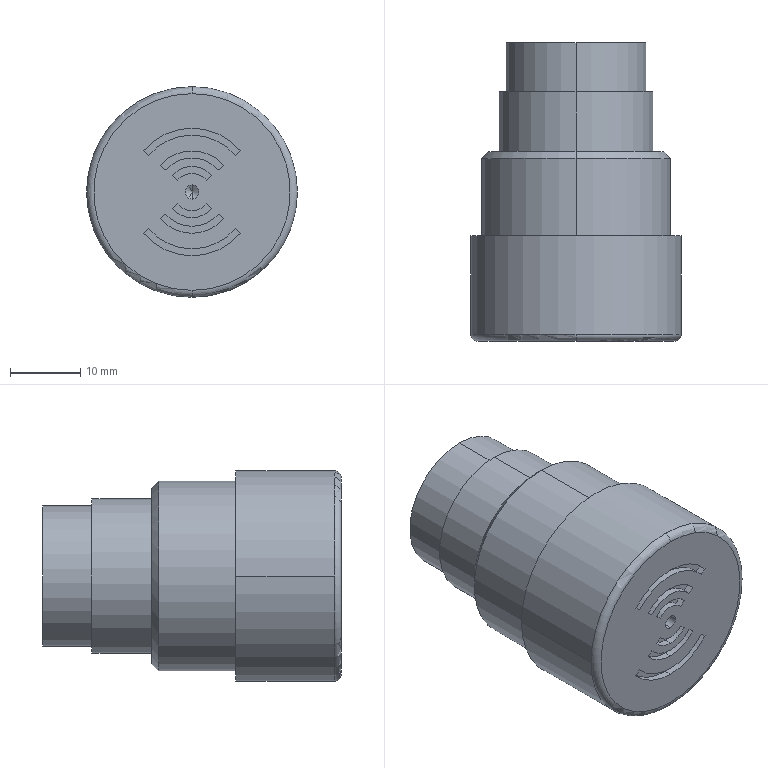Part | SolidWorks | features ICE 2, BaseBody 1, CutThin 1, Fillet 1, HoleWzd 1 | 1 solid | 60 faces | box 30 x 42.5 x 30 mm | volume 22012 mm3 | cylinder 30 | plane 24 | cone 4 | torus 2 | commonest cylinder face diameters 5.299 x3 7.299 x3 9.752 x3 11.752 x3 16.175 x3 18.175 x3